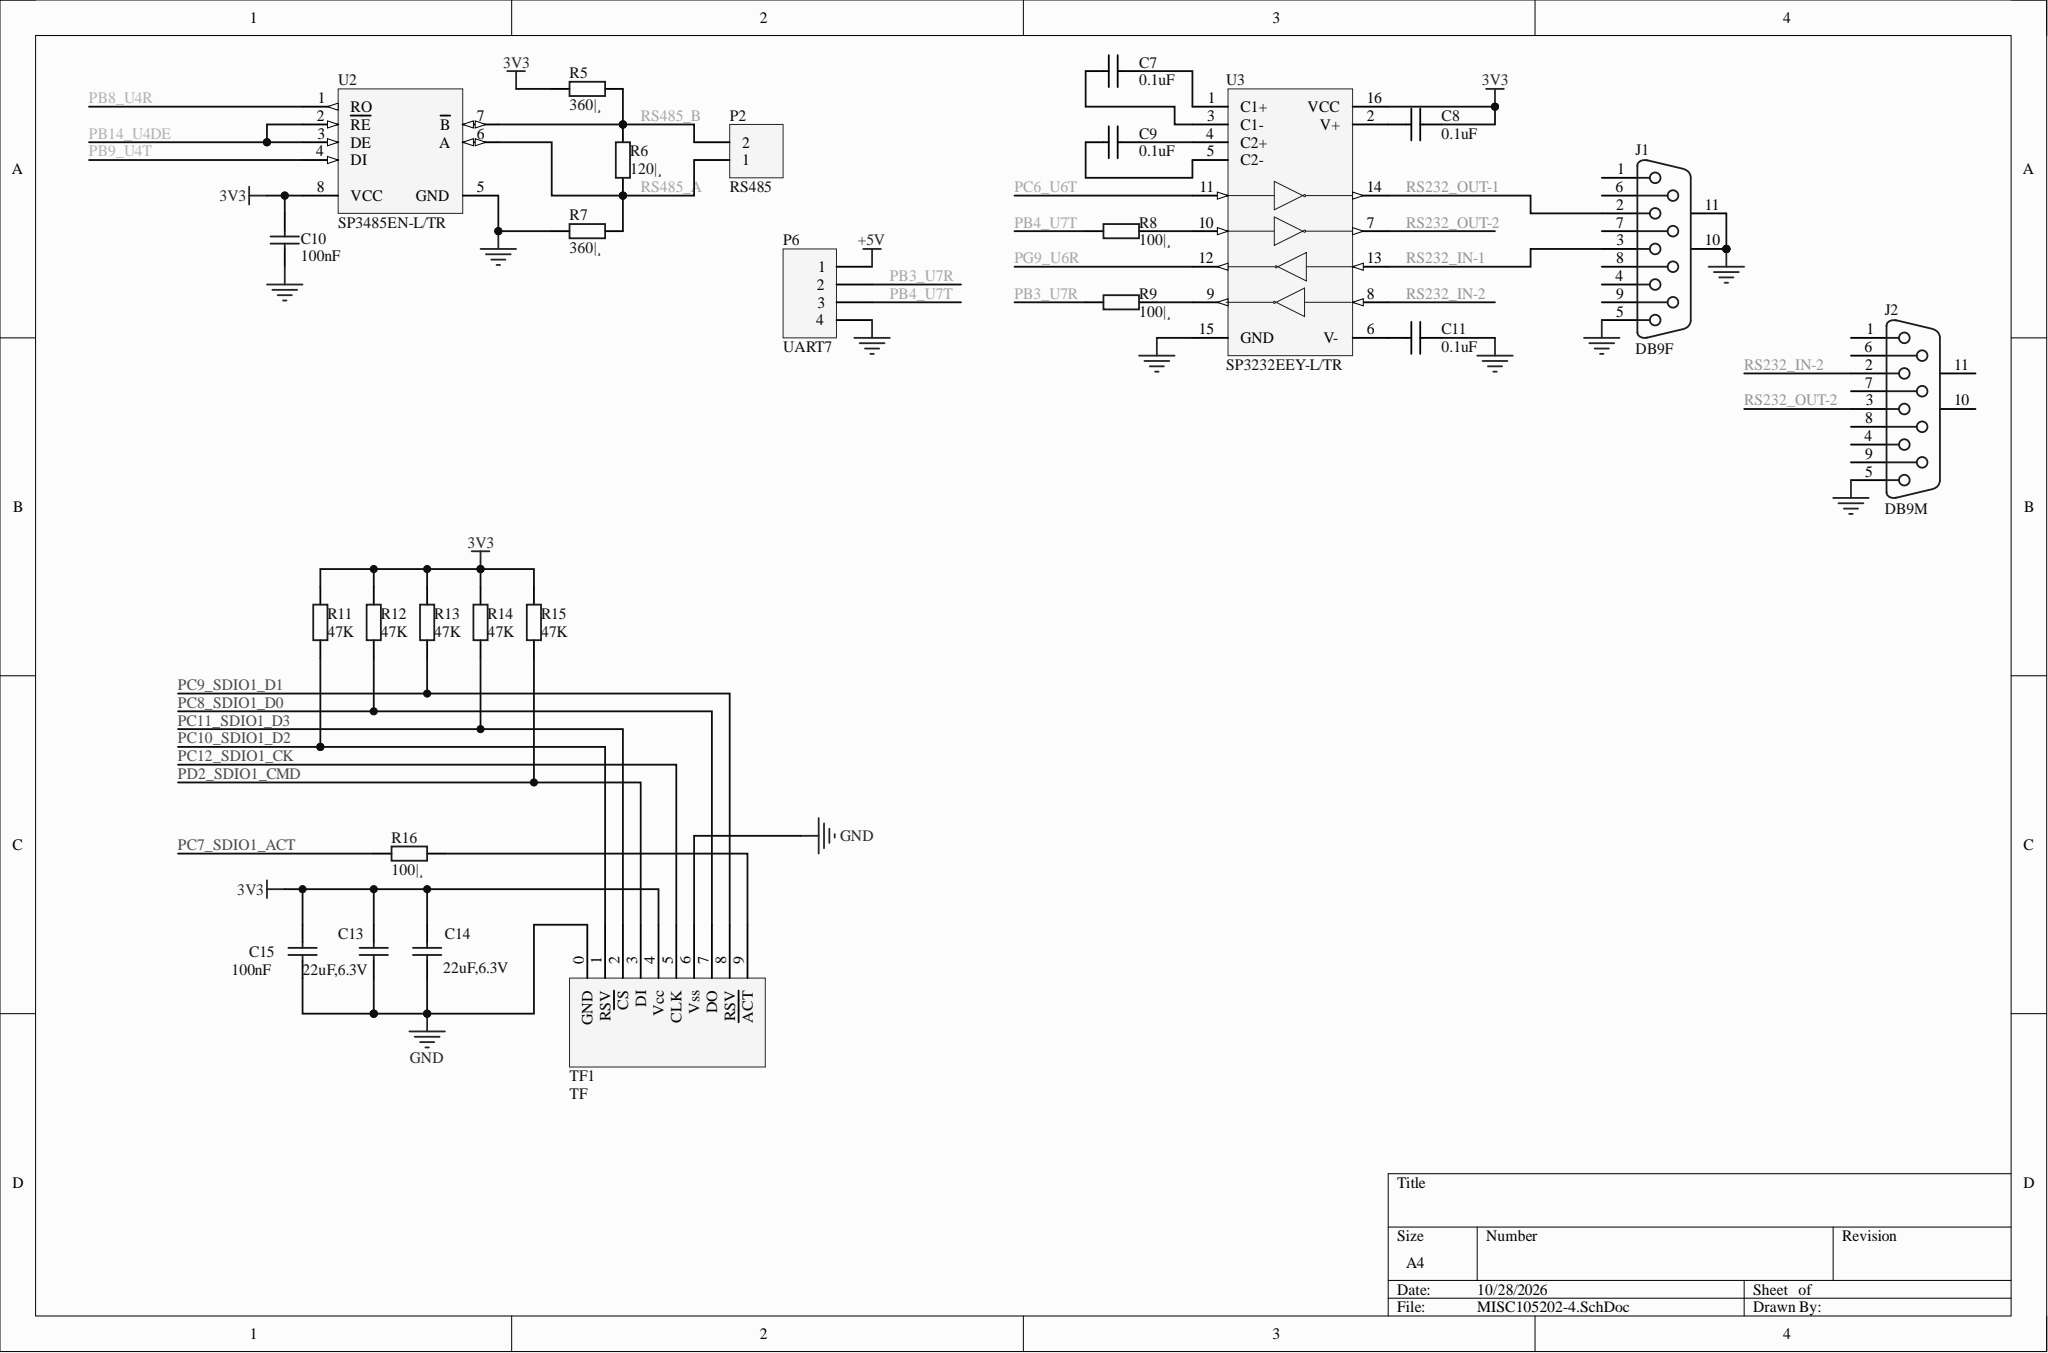Circuit board | Altium Designer | 181 parts | 141 nets | one sheet of the schematic
Parts on this sheet (reference | value | footprint):
C7 | 0.1uF | 0603_C
C8 | 0.1uF | 0603_C
C9 | 0.1uF | 0603_C
C10 | 100nF | 0603_C
C11 | 0.1uF | 0603_C
C13 | 22uF,6.3V | 0603_C
C14 | 22uF,6.3V | 0603_C
C15 | 100nF | 0402_C
J1 | DB9F | DB9RA/F
J2 | DB9M | DB9RA/M
P2 | RS485 | 508*2B
P6 | UART7 | HDR1X4
R5 | 360|¸ | 0603_R
R6 | 120|¸ | 0603_R
R7 | 360|¸ | 0603_R
R8 | 100|¸ | 0603_R
R9 | 100|¸ | 0603_R
R11 | 47K | 0402_R
R12 | 47K | 0402_R
R13 | 47K | 0402_R
R14 | 47K | 0402_R
R15 | 47K | 0402_R
R16 | 100|¸ | 0402_R
TF1 | TF | MICROSD
U2 | SP3485EN-L/TR | SOIC-8_150mil
U3 | SP3232EEY-L/TR | TSSOP-16
Nets of these parts (net: part-pin ...):
RS485_B: P2-2 R5-2 R6-1 U2-7
RS485_A: P2-1 R6-2 R7-2 U2-6
RS232_OUT-2: J2-3 U3-7
RS232_OUT-1: J1-2 U3-14
RS232_IN-2: J2-2 U3-8
RS232_IN-1: J1-3 U3-13
PG9_QSPI_BK2_IO2: U3-12
PD2_SDIO1_CMD: R15-1 TF1-3
PC12_SDIO1_CK: TF1-5
PC11_SDIO1_D3: R14-1 TF1-2
PC10_SDIO1_D2: R11-1 TF1-1
PC9_SDIO1_D1: R13-1 TF1-8
PC8_SDIO1_D0: R12-1 TF1-7
PC7_SDIO1_ACT: R16-1
PC6_SDIO1_D0DIR: U3-11
PB14_SDIO2_D0: U2-2 U2-3
PB9_SDIO1_CDIR: U2-4
PB8_SDIO1_CKIN: U2-1
PB4_SDIO2_D3: P6-3 R8-1
PB3_SDIO2_D2: P6-2 R9-1
NetR16_2: R16-2 TF1-9
NetR9_2: R9-2 U3-9
NetR8_2: R8-2 U3-10
NetC11_2: C11-2 U3-6
NetC9_2: C9-2 U3-5
NetC9_1: C9-1 U3-4
NetC8_2: C8-2 U3-2
NetC7_2: C7-2 U3-3
NetC7_1: C7-1 U3-1
GND: C10-1 C11-1 C13-1 C14-1 C15-1 J1-5 J1-10 J1-11 J2-5 P6-4 R7-1 TF1-0 TF1-6 U2-5 U3-15
+5V: P6-1
3V3: C8-1 C10-2 C13-2 C14-2 C15-2 R5-1 R11-2 R12-2 R13-2 R14-2 R15-2 TF1-4 U2-8 U3-16